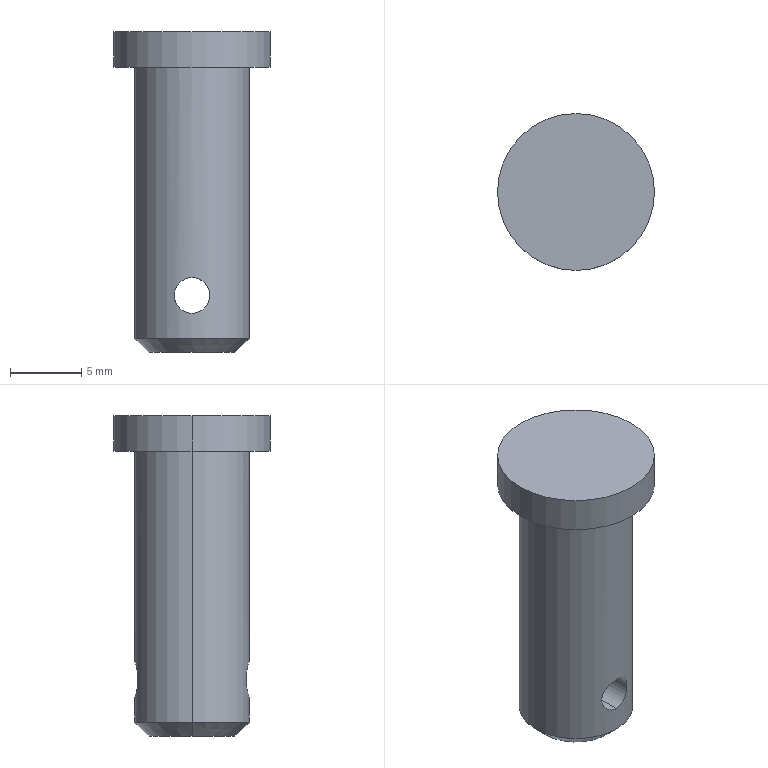Part | NX | features BREP 1 | 1 solid | 11 faces | box 11 x 11 x 22.5 mm | volume 1193 mm3 | cylinder 6 | plane 3 | cone 2 | commonest cylinder face diameters 2.5 x2 8 x2 11 x2
STEP:
#1=CARTESIAN_POINT('',(5.5,0.,20.));
#2=VERTEX_POINT('',#1);
#3=CARTESIAN_POINT('',(5.5,0.,22.5));
#4=VERTEX_POINT('',#3);
#5=CARTESIAN_POINT('',(5.5,0.,20.));
#6=DIRECTION('',(0.,0.,1.));
#7=VECTOR('',#6,1000.);
#8=LINE('',#5,#7);
#9=EDGE_CURVE('',#2,#4,#8,.T.);
#10=ORIENTED_EDGE('',*,*,#9,.F.);
#11=CARTESIAN_POINT('',(-5.5,0.,20.));
#12=VERTEX_POINT('',#11);
#13=CARTESIAN_POINT('',(0.,0.,20.));
#14=DIRECTION('',(0.,0.,-1.));
#15=DIRECTION('',(-1.,0.,0.));
#16=AXIS2_PLACEMENT_3D('',#13,#14,#15);
#17=CIRCLE('',#16,5.5);
#18=EDGE_CURVE('',#12,#2,#17,.T.);
#19=ORIENTED_EDGE('',*,*,#18,.F.);
#20=CARTESIAN_POINT('',(-5.5,0.,22.5));
#21=VERTEX_POINT('',#20);
#22=CARTESIAN_POINT('',(-5.5,0.,20.));
#23=DIRECTION('',(0.,0.,1.));
#24=VECTOR('',#23,1000.);
#25=LINE('',#22,#24);
#26=EDGE_CURVE('',#12,#21,#25,.T.);
#27=ORIENTED_EDGE('',*,*,#26,.T.);
#28=CARTESIAN_POINT('',(0.,0.,22.5));
#29=DIRECTION('',(0.,0.,1.));
#30=DIRECTION('',(1.,0.,0.));
#31=AXIS2_PLACEMENT_3D('',#28,#29,#30);
#32=CIRCLE('',#31,5.5);
#33=EDGE_CURVE('',#4,#21,#32,.T.);
#34=ORIENTED_EDGE('',*,*,#33,.F.);
#35=EDGE_LOOP('',(#10,#19,#27,#34));
#36=FACE_BOUND('',#35,.T.);
#37=CARTESIAN_POINT('',(0.,0.,22.5));
#38=DIRECTION('',(0.,0.,-1.));
#39=DIRECTION('',(1.,0.,0.));
#40=AXIS2_PLACEMENT_3D('',#37,#38,#39);
#41=CYLINDRICAL_SURFACE('',#40,5.5);
#42=ADVANCED_FACE('',(#36),#41,.T.);
#43=ORIENTED_EDGE('',*,*,#33,.T.);
#44=CARTESIAN_POINT('',(0.,0.,22.5));
#45=DIRECTION('',(0.,0.,1.));
#46=DIRECTION('',(-1.,0.,0.));
#47=AXIS2_PLACEMENT_3D('',#44,#45,#46);
#48=CIRCLE('',#47,5.5);
#49=EDGE_CURVE('',#21,#4,#48,.T.);
#50=ORIENTED_EDGE('',*,*,#49,.T.);
#51=EDGE_LOOP('',(#43,#50));
#52=FACE_BOUND('',#51,.T.);
#53=CARTESIAN_POINT('',(0.,0.,22.5));
#54=DIRECTION('',(0.,0.,1.));
#55=DIRECTION('',(-1.,0.,0.));
#56=AXIS2_PLACEMENT_3D('',#53,#54,#55);
#57=PLANE('',#56);
#58=ADVANCED_FACE('',(#52),#57,.T.);
#59=ORIENTED_EDGE('',*,*,#49,.F.);
#60=ORIENTED_EDGE('',*,*,#26,.F.);
#61=CARTESIAN_POINT('',(0.,0.,20.));
#62=DIRECTION('',(0.,0.,-1.));
#63=DIRECTION('',(1.,0.,0.));
#64=AXIS2_PLACEMENT_3D('',#61,#62,#63);
#65=CIRCLE('',#64,5.5);
#66=EDGE_CURVE('',#2,#12,#65,.T.);
#67=ORIENTED_EDGE('',*,*,#66,.F.);
#68=ORIENTED_EDGE('',*,*,#9,.T.);
#69=EDGE_LOOP('',(#59,#60,#67,#68));
#70=FACE_BOUND('',#69,.T.);
#71=CARTESIAN_POINT('',(0.,0.,22.5));
#72=DIRECTION('',(0.,0.,-1.));
#73=DIRECTION('',(1.,0.,0.));
#74=AXIS2_PLACEMENT_3D('',#71,#72,#73);
#75=CYLINDRICAL_SURFACE('',#74,5.5);
#76=ADVANCED_FACE('',(#70),#75,.T.);
#77=ORIENTED_EDGE('',*,*,#18,.T.);
#78=ORIENTED_EDGE('',*,*,#66,.T.);
#79=EDGE_LOOP('',(#77,#78));
#80=FACE_BOUND('',#79,.T.);
#81=CARTESIAN_POINT('',(4.,0.,20.));
#82=VERTEX_POINT('',#81);
#83=CARTESIAN_POINT('',(-4.,0.,20.));
#84=VERTEX_POINT('',#83);
#85=CARTESIAN_POINT('',(0.,0.,20.));
#86=DIRECTION('',(0.,0.,1.));
#87=DIRECTION('',(1.,0.,0.));
#88=AXIS2_PLACEMENT_3D('',#85,#86,#87);
#89=CIRCLE('',#88,4.);
#90=EDGE_CURVE('',#82,#84,#89,.T.);
#91=ORIENTED_EDGE('',*,*,#90,.T.);
#92=CARTESIAN_POINT('',(0.,0.,20.));
#93=DIRECTION('',(0.,0.,1.));
#94=DIRECTION('',(-1.,0.,0.));
#95=AXIS2_PLACEMENT_3D('',#92,#93,#94);
#96=CIRCLE('',#95,4.);
#97=EDGE_CURVE('',#84,#82,#96,.T.);
#98=ORIENTED_EDGE('',*,*,#97,.T.);
#99=EDGE_LOOP('',(#91,#98));
#100=FACE_BOUND('',#99,.T.);
#101=CARTESIAN_POINT('',(0.,0.,20.));
#102=DIRECTION('',(0.,0.,1.));
#103=DIRECTION('',(-1.,0.,0.));
#104=AXIS2_PLACEMENT_3D('',#101,#102,#103);
#105=PLANE('',#104);
#106=ADVANCED_FACE('',(#80,#100),#105,.F.);
#107=ORIENTED_EDGE('',*,*,#97,.F.);
#108=CARTESIAN_POINT('',(-4.,0.,1.));
#109=VERTEX_POINT('',#108);
#110=CARTESIAN_POINT('',(-4.,0.,1.));
#111=DIRECTION('',(0.,0.,1.));
#112=VECTOR('',#111,1000.);
#113=LINE('',#110,#112);
#114=EDGE_CURVE('',#84,#109,#113,.F.);
#115=ORIENTED_EDGE('',*,*,#114,.T.);
#116=CARTESIAN_POINT('',(4.,0.,1.));
#117=VERTEX_POINT('',#116);
#118=CARTESIAN_POINT('',(0.,0.,1.));
#119=DIRECTION('',(0.,0.,-1.));
#120=DIRECTION('',(1.,0.,0.));
#121=AXIS2_PLACEMENT_3D('',#118,#119,#120);
#122=CIRCLE('',#121,4.);
#123=EDGE_CURVE('',#117,#109,#122,.T.);
#124=ORIENTED_EDGE('',*,*,#123,.F.);
#125=CARTESIAN_POINT('',(4.,0.,1.));
#126=DIRECTION('',(0.,0.,1.));
#127=VECTOR('',#126,1000.);
#128=LINE('',#125,#127);
#129=EDGE_CURVE('',#82,#117,#128,.F.);
#130=ORIENTED_EDGE('',*,*,#129,.F.);
#131=EDGE_LOOP('',(#107,#115,#124,#130));
#132=FACE_BOUND('',#131,.T.);
#133=CARTESIAN_POINT('',(0.,-4.,5.25));
#134=VERTEX_POINT('',#133);
#135=CARTESIAN_POINT('',(0.,-4.,2.75));
#136=VERTEX_POINT('',#135);
#137=CARTESIAN_POINT('',(0.,-4.,5.25));
#138=CARTESIAN_POINT('',(-0.3325,-4.,5.25));
#139=CARTESIAN_POINT('',(-0.9768,-3.902,4.979));
#140=CARTESIAN_POINT('',(-1.386,-3.748,4.002));
#141=CARTESIAN_POINT('',(-0.9773,-3.902,3.021));
#142=CARTESIAN_POINT('',(-0.3325,-4.,2.75));
#143=CARTESIAN_POINT('',(0.,-4.,2.75));
#144=B_SPLINE_CURVE_WITH_KNOTS('',3,(#137,#138,#139,#140,#141,#142,#143),.UNSPECIFIED.,.F.,.F.,(4,1,1,1,4),(0.,0.0009829,0.001966,0.002949,0.003931),.UNSPECIFIED.);
#145=EDGE_CURVE('',#134,#136,#144,.T.);
#146=ORIENTED_EDGE('',*,*,#145,.F.);
#147=CARTESIAN_POINT('',(0.,-4.,2.75));
#148=CARTESIAN_POINT('',(0.3325,-4.,2.75));
#149=CARTESIAN_POINT('',(0.9768,-3.902,3.021));
#150=CARTESIAN_POINT('',(1.386,-3.748,3.998));
#151=CARTESIAN_POINT('',(0.9773,-3.902,4.979));
#152=CARTESIAN_POINT('',(0.3325,-4.,5.25));
#153=CARTESIAN_POINT('',(0.,-4.,5.25));
#154=B_SPLINE_CURVE_WITH_KNOTS('',3,(#147,#148,#149,#150,#151,#152,#153),.UNSPECIFIED.,.F.,.F.,(4,1,1,1,4),(0.,0.0009829,0.001966,0.002949,0.003931),.UNSPECIFIED.);
#155=EDGE_CURVE('',#136,#134,#154,.T.);
#156=ORIENTED_EDGE('',*,*,#155,.F.);
#157=EDGE_LOOP('',(#146,#156));
#158=FACE_BOUND('',#157,.T.);
#159=CARTESIAN_POINT('',(0.,0.,20.));
#160=DIRECTION('',(0.,0.,-1.));
#161=DIRECTION('',(1.,0.,0.));
#162=AXIS2_PLACEMENT_3D('',#159,#160,#161);
#163=CYLINDRICAL_SURFACE('',#162,4.);
#164=ADVANCED_FACE('',(#132,#158),#163,.T.);
#165=ORIENTED_EDGE('',*,*,#129,.T.);
#166=CARTESIAN_POINT('',(0.,0.,1.));
#167=DIRECTION('',(0.,0.,-1.));
#168=DIRECTION('',(-1.,0.,0.));
#169=AXIS2_PLACEMENT_3D('',#166,#167,#168);
#170=CIRCLE('',#169,4.);
#171=EDGE_CURVE('',#109,#117,#170,.T.);
#172=ORIENTED_EDGE('',*,*,#171,.F.);
#173=ORIENTED_EDGE('',*,*,#114,.F.);
#174=ORIENTED_EDGE('',*,*,#90,.F.);
#175=EDGE_LOOP('',(#165,#172,#173,#174));
#176=FACE_BOUND('',#175,.T.);
#177=CARTESIAN_POINT('',(0.,4.,5.25));
#178=VERTEX_POINT('',#177);
#179=CARTESIAN_POINT('',(0.,4.,2.75));
#180=VERTEX_POINT('',#179);
#181=CARTESIAN_POINT('',(0.,4.,5.25));
#182=CARTESIAN_POINT('',(0.3325,4.,5.25));
#183=CARTESIAN_POINT('',(0.9768,3.902,4.979));
#184=CARTESIAN_POINT('',(1.386,3.748,4.002));
#185=CARTESIAN_POINT('',(0.9773,3.902,3.021));
#186=CARTESIAN_POINT('',(0.3325,4.,2.75));
#187=CARTESIAN_POINT('',(0.,4.,2.75));
#188=B_SPLINE_CURVE_WITH_KNOTS('',3,(#181,#182,#183,#184,#185,#186,#187),.UNSPECIFIED.,.F.,.F.,(4,1,1,1,4),(0.,0.0009829,0.001966,0.002949,0.003931),.UNSPECIFIED.);
#189=EDGE_CURVE('',#178,#180,#188,.T.);
#190=ORIENTED_EDGE('',*,*,#189,.F.);
#191=CARTESIAN_POINT('',(0.,4.,2.75));
#192=CARTESIAN_POINT('',(-0.3325,4.,2.75));
#193=CARTESIAN_POINT('',(-0.9768,3.902,3.021));
#194=CARTESIAN_POINT('',(-1.386,3.748,3.998));
#195=CARTESIAN_POINT('',(-0.9773,3.902,4.979));
#196=CARTESIAN_POINT('',(-0.3325,4.,5.25));
#197=CARTESIAN_POINT('',(0.,4.,5.25));
#198=B_SPLINE_CURVE_WITH_KNOTS('',3,(#191,#192,#193,#194,#195,#196,#197),.UNSPECIFIED.,.F.,.F.,(4,1,1,1,4),(0.,0.0009829,0.001966,0.002949,0.003931),.UNSPECIFIED.);
#199=EDGE_CURVE('',#180,#178,#198,.T.);
#200=ORIENTED_EDGE('',*,*,#199,.F.);
#201=EDGE_LOOP('',(#190,#200));
#202=FACE_BOUND('',#201,.T.);
#203=CARTESIAN_POINT('',(0.,0.,20.));
#204=DIRECTION('',(0.,0.,-1.));
#205=DIRECTION('',(1.,0.,0.));
#206=AXIS2_PLACEMENT_3D('',#203,#204,#205);
#207=CYLINDRICAL_SURFACE('',#206,4.);
#208=ADVANCED_FACE('',(#176,#202),#207,.T.);
#209=CARTESIAN_POINT('',(-3.,0.,0.));
#210=VERTEX_POINT('',#209);
#211=CARTESIAN_POINT('',(-4.,0.,1.));
#212=DIRECTION('',(0.7071,0.,-0.7071));
#213=VECTOR('',#212,1000.);
#214=LINE('',#211,#213);
#215=EDGE_CURVE('',#210,#109,#214,.F.);
#216=ORIENTED_EDGE('',*,*,#215,.T.);
#217=ORIENTED_EDGE('',*,*,#171,.T.);
#218=CARTESIAN_POINT('',(3.,0.,0.));
#219=VERTEX_POINT('',#218);
#220=CARTESIAN_POINT('',(4.,0.,1.));
#221=DIRECTION('',(-0.7071,0.,-0.7071));
#222=VECTOR('',#221,1000.);
#223=LINE('',#220,#222);
#224=EDGE_CURVE('',#219,#117,#223,.F.);
#225=ORIENTED_EDGE('',*,*,#224,.F.);
#226=CARTESIAN_POINT('',(0.,0.,0.));
#227=DIRECTION('',(0.,0.,-1.));
#228=DIRECTION('',(-1.,0.,0.));
#229=AXIS2_PLACEMENT_3D('',#226,#227,#228);
#230=CIRCLE('',#229,3.);
#231=EDGE_CURVE('',#210,#219,#230,.T.);
#232=ORIENTED_EDGE('',*,*,#231,.F.);
#233=EDGE_LOOP('',(#216,#217,#225,#232));
#234=FACE_BOUND('',#233,.T.);
#235=CARTESIAN_POINT('',(0.,0.,0.5));
#236=DIRECTION('',(0.,0.,1.));
#237=DIRECTION('',(-1.,0.,0.));
#238=AXIS2_PLACEMENT_3D('',#235,#236,#237);
#239=CONICAL_SURFACE('',#238,3.5,0.7854);
#240=ADVANCED_FACE('',(#234),#239,.T.);
#241=ORIENTED_EDGE('',*,*,#231,.T.);
#242=CARTESIAN_POINT('',(0.,0.,0.));
#243=DIRECTION('',(0.,0.,-1.));
#244=DIRECTION('',(1.,0.,0.));
#245=AXIS2_PLACEMENT_3D('',#242,#243,#244);
#246=CIRCLE('',#245,3.);
#247=EDGE_CURVE('',#219,#210,#246,.T.);
#248=ORIENTED_EDGE('',*,*,#247,.T.);
#249=EDGE_LOOP('',(#241,#248));
#250=FACE_BOUND('',#249,.T.);
#251=CARTESIAN_POINT('',(0.,0.,0.));
#252=DIRECTION('',(0.,0.,1.));
#253=DIRECTION('',(-1.,0.,0.));
#254=AXIS2_PLACEMENT_3D('',#251,#252,#253);
#255=PLANE('',#254);
#256=ADVANCED_FACE('',(#250),#255,.F.);
#257=ORIENTED_EDGE('',*,*,#247,.F.);
#258=ORIENTED_EDGE('',*,*,#224,.T.);
#259=ORIENTED_EDGE('',*,*,#123,.T.);
#260=ORIENTED_EDGE('',*,*,#215,.F.);
#261=EDGE_LOOP('',(#257,#258,#259,#260));
#262=FACE_BOUND('',#261,.T.);
#263=CARTESIAN_POINT('',(0.,0.,0.5));
#264=DIRECTION('',(0.,0.,1.));
#265=DIRECTION('',(-1.,0.,0.));
#266=AXIS2_PLACEMENT_3D('',#263,#264,#265);
#267=CONICAL_SURFACE('',#266,3.5,0.7854);
#268=ADVANCED_FACE('',(#262),#267,.T.);
#269=CARTESIAN_POINT('',(0.,4.,2.75));
#270=DIRECTION('',(0.,-1.,0.));
#271=VECTOR('',#270,1000.);
#272=LINE('',#269,#271);
#273=EDGE_CURVE('',#136,#180,#272,.F.);
#274=ORIENTED_EDGE('',*,*,#273,.T.);
#275=ORIENTED_EDGE('',*,*,#199,.T.);
#276=CARTESIAN_POINT('',(0.,4.,5.25));
#277=DIRECTION('',(0.,-1.,0.));
#278=VECTOR('',#277,1000.);
#279=LINE('',#276,#278);
#280=EDGE_CURVE('',#134,#178,#279,.F.);
#281=ORIENTED_EDGE('',*,*,#280,.F.);
#282=ORIENTED_EDGE('',*,*,#145,.T.);
#283=EDGE_LOOP('',(#274,#275,#281,#282));
#284=FACE_BOUND('',#283,.T.);
#285=CARTESIAN_POINT('',(0.,-6.25,4.));
#286=DIRECTION('',(0.,1.,0.));
#287=DIRECTION('',(0.,0.,-1.));
#288=AXIS2_PLACEMENT_3D('',#285,#286,#287);
#289=CYLINDRICAL_SURFACE('',#288,1.25);
#290=ADVANCED_FACE('',(#284),#289,.F.);
#291=ORIENTED_EDGE('',*,*,#155,.T.);
#292=ORIENTED_EDGE('',*,*,#280,.T.);
#293=ORIENTED_EDGE('',*,*,#189,.T.);
#294=ORIENTED_EDGE('',*,*,#273,.F.);
#295=EDGE_LOOP('',(#291,#292,#293,#294));
#296=FACE_BOUND('',#295,.T.);
#297=CARTESIAN_POINT('',(0.,-6.25,4.));
#298=DIRECTION('',(0.,1.,0.));
#299=DIRECTION('',(0.,0.,-1.));
#300=AXIS2_PLACEMENT_3D('',#297,#298,#299);
#301=CYLINDRICAL_SURFACE('',#300,1.25);
#302=ADVANCED_FACE('',(#296),#301,.F.);
#303=CLOSED_SHELL('',(#42,#58,#76,#106,#164,#208,#240,#256,#268,#290,#302));
#304=MANIFOLD_SOLID_BREP('',#303);
#305=(LENGTH_UNIT()NAMED_UNIT(*)SI_UNIT(.MILLI.,.METRE.));
#306=UNCERTAINTY_MEASURE_WITH_UNIT(LENGTH_MEASURE(0.0508),#305,'','');
#307=(NAMED_UNIT(*)PLANE_ANGLE_UNIT()SI_UNIT($,.RADIAN.));
#308=(NAMED_UNIT(*)SI_UNIT($,.STERADIAN.)SOLID_ANGLE_UNIT());
#309=(GEOMETRIC_REPRESENTATION_CONTEXT(3)GLOBAL_UNCERTAINTY_ASSIGNED_CONTEXT((#306))GLOBAL_UNIT_ASSIGNED_CONTEXT((#305,#307,#308))REPRESENTATION_CONTEXT('',''));
#310=ADVANCED_BREP_SHAPE_REPRESENTATION('',(#304),#309);